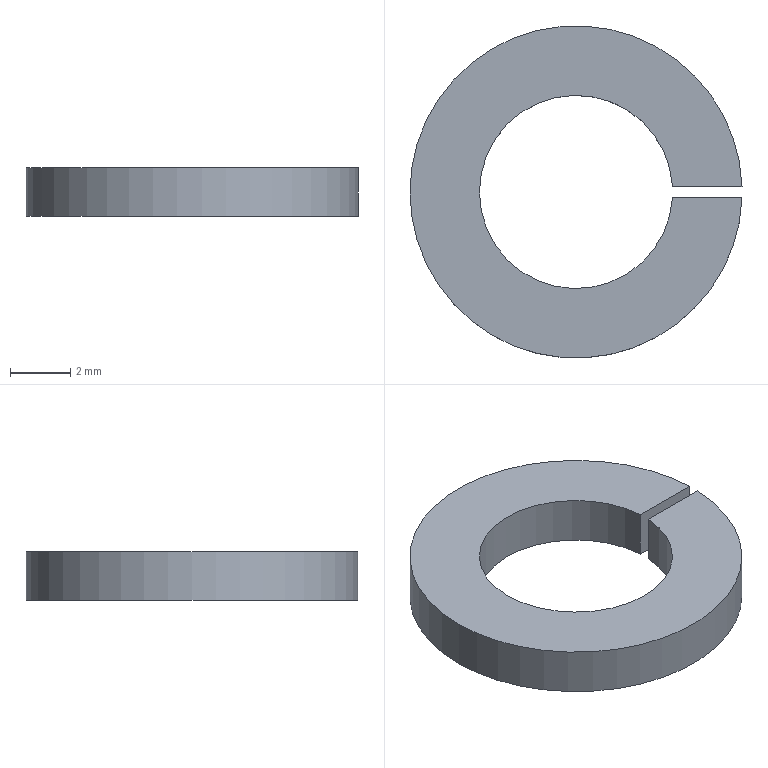Part | STEP file | GB93-1987 washer 6 | 1 solid | 6 faces | box 10.997 x 11 x 1.6 mm | volume 99.231 mm3 | plane 4 | cylinder 2 | commonest cylinder face diameters 6.4 x1 11 x1
STEP:
#1=CARTESIAN_POINT('',(5.497,0.1833,1.6));
#2=VERTEX_POINT('',#1);
#3=CARTESIAN_POINT('',(5.497,-0.1833,1.6));
#4=VERTEX_POINT('',#3);
#5=CARTESIAN_POINT('',(0.,0.,1.6));
#6=DIRECTION('',(0.,0.,1.));
#7=DIRECTION('',(1.,0.,0.));
#8=AXIS2_PLACEMENT_3D('',#5,#6,#7);
#9=CIRCLE('',#8,5.5);
#10=EDGE_CURVE('',#2,#4,#9,.T.);
#11=ORIENTED_EDGE('',*,*,#10,.T.);
#12=CARTESIAN_POINT('',(3.195,-0.1833,1.6));
#13=VERTEX_POINT('',#12);
#14=CARTESIAN_POINT('',(0.,-0.1833,1.6));
#15=DIRECTION('',(1.,0.,0.));
#16=VECTOR('',#15,1000.);
#17=LINE('',#14,#16);
#18=EDGE_CURVE('',#13,#4,#17,.T.);
#19=ORIENTED_EDGE('',*,*,#18,.F.);
#20=CARTESIAN_POINT('',(3.195,0.1833,1.6));
#21=VERTEX_POINT('',#20);
#22=CARTESIAN_POINT('',(0.,0.,1.6));
#23=DIRECTION('',(0.,0.,1.));
#24=DIRECTION('',(1.,0.,0.));
#25=AXIS2_PLACEMENT_3D('',#22,#23,#24);
#26=CIRCLE('',#25,3.2);
#27=EDGE_CURVE('',#21,#13,#26,.T.);
#28=ORIENTED_EDGE('',*,*,#27,.F.);
#29=CARTESIAN_POINT('',(0.,0.1833,1.6));
#30=DIRECTION('',(-1.,0.,0.));
#31=VECTOR('',#30,1000.);
#32=LINE('',#29,#31);
#33=EDGE_CURVE('',#2,#21,#32,.T.);
#34=ORIENTED_EDGE('',*,*,#33,.F.);
#35=EDGE_LOOP('',(#11,#19,#28,#34));
#36=FACE_OUTER_BOUND('',#35,.T.);
#37=CARTESIAN_POINT('',(0.,0.,1.6));
#38=DIRECTION('',(0.,0.,1.));
#39=DIRECTION('',(1.,0.,0.));
#40=AXIS2_PLACEMENT_3D('',#37,#38,#39);
#41=PLANE('',#40);
#42=ADVANCED_FACE('',(#36),#41,.T.);
#43=CARTESIAN_POINT('',(3.195,-0.1833,0.));
#44=VERTEX_POINT('',#43);
#45=CARTESIAN_POINT('',(5.497,-0.1833,0.));
#46=VERTEX_POINT('',#45);
#47=CARTESIAN_POINT('',(0.,-0.1833,0.));
#48=DIRECTION('',(1.,0.,0.));
#49=VECTOR('',#48,1000.);
#50=LINE('',#47,#49);
#51=EDGE_CURVE('',#44,#46,#50,.T.);
#52=ORIENTED_EDGE('',*,*,#51,.T.);
#53=CARTESIAN_POINT('',(5.497,0.1833,0.));
#54=VERTEX_POINT('',#53);
#55=CARTESIAN_POINT('',(0.,0.,0.));
#56=DIRECTION('',(0.,0.,1.));
#57=DIRECTION('',(1.,0.,0.));
#58=AXIS2_PLACEMENT_3D('',#55,#56,#57);
#59=CIRCLE('',#58,5.5);
#60=EDGE_CURVE('',#54,#46,#59,.T.);
#61=ORIENTED_EDGE('',*,*,#60,.F.);
#62=CARTESIAN_POINT('',(3.195,0.1833,0.));
#63=VERTEX_POINT('',#62);
#64=CARTESIAN_POINT('',(0.,0.1833,0.));
#65=DIRECTION('',(-1.,0.,0.));
#66=VECTOR('',#65,1000.);
#67=LINE('',#64,#66);
#68=EDGE_CURVE('',#54,#63,#67,.T.);
#69=ORIENTED_EDGE('',*,*,#68,.T.);
#70=CARTESIAN_POINT('',(0.,0.,0.));
#71=DIRECTION('',(0.,0.,1.));
#72=DIRECTION('',(1.,0.,0.));
#73=AXIS2_PLACEMENT_3D('',#70,#71,#72);
#74=CIRCLE('',#73,3.2);
#75=EDGE_CURVE('',#63,#44,#74,.T.);
#76=ORIENTED_EDGE('',*,*,#75,.T.);
#77=EDGE_LOOP('',(#52,#61,#69,#76));
#78=FACE_OUTER_BOUND('',#77,.T.);
#79=CARTESIAN_POINT('',(0.,0.,0.));
#80=DIRECTION('',(0.,0.,1.));
#81=DIRECTION('',(1.,0.,0.));
#82=AXIS2_PLACEMENT_3D('',#79,#80,#81);
#83=PLANE('',#82);
#84=ADVANCED_FACE('',(#78),#83,.F.);
#85=CARTESIAN_POINT('',(5.497,-0.1833,1.6));
#86=DIRECTION('',(0.,0.,-1.));
#87=VECTOR('',#86,1000.);
#88=LINE('',#85,#87);
#89=EDGE_CURVE('',#4,#46,#88,.T.);
#90=ORIENTED_EDGE('',*,*,#89,.F.);
#91=ORIENTED_EDGE('',*,*,#10,.F.);
#92=CARTESIAN_POINT('',(5.497,0.1833,1.6));
#93=DIRECTION('',(0.,0.,1.));
#94=VECTOR('',#93,1000.);
#95=LINE('',#92,#94);
#96=EDGE_CURVE('',#54,#2,#95,.T.);
#97=ORIENTED_EDGE('',*,*,#96,.F.);
#98=ORIENTED_EDGE('',*,*,#60,.T.);
#99=EDGE_LOOP('',(#90,#91,#97,#98));
#100=FACE_OUTER_BOUND('',#99,.T.);
#101=CARTESIAN_POINT('',(0.,0.,1.6));
#102=DIRECTION('',(0.,0.,-1.));
#103=DIRECTION('',(-1.,0.,0.));
#104=AXIS2_PLACEMENT_3D('',#101,#102,#103);
#105=CYLINDRICAL_SURFACE('',#104,5.5);
#106=ADVANCED_FACE('',(#100),#105,.T.);
#107=ORIENTED_EDGE('',*,*,#27,.T.);
#108=CARTESIAN_POINT('',(3.195,-0.1833,1.6));
#109=DIRECTION('',(0.,0.,-1.));
#110=VECTOR('',#109,1000.);
#111=LINE('',#108,#110);
#112=EDGE_CURVE('',#13,#44,#111,.T.);
#113=ORIENTED_EDGE('',*,*,#112,.T.);
#114=ORIENTED_EDGE('',*,*,#75,.F.);
#115=CARTESIAN_POINT('',(3.195,0.1833,1.6));
#116=DIRECTION('',(0.,0.,1.));
#117=VECTOR('',#116,1000.);
#118=LINE('',#115,#117);
#119=EDGE_CURVE('',#63,#21,#118,.T.);
#120=ORIENTED_EDGE('',*,*,#119,.T.);
#121=EDGE_LOOP('',(#107,#113,#114,#120));
#122=FACE_OUTER_BOUND('',#121,.T.);
#123=CARTESIAN_POINT('',(0.,0.,1.6));
#124=DIRECTION('',(0.,0.,-1.));
#125=DIRECTION('',(-1.,0.,0.));
#126=AXIS2_PLACEMENT_3D('',#123,#124,#125);
#127=CYLINDRICAL_SURFACE('',#126,3.2);
#128=ADVANCED_FACE('',(#122),#127,.F.);
#129=ORIENTED_EDGE('',*,*,#96,.T.);
#130=ORIENTED_EDGE('',*,*,#33,.T.);
#131=ORIENTED_EDGE('',*,*,#119,.F.);
#132=ORIENTED_EDGE('',*,*,#68,.F.);
#133=EDGE_LOOP('',(#129,#130,#131,#132));
#134=FACE_OUTER_BOUND('',#133,.T.);
#135=CARTESIAN_POINT('',(0.,0.1833,1.6));
#136=DIRECTION('',(0.,-1.,0.));
#137=DIRECTION('',(0.,0.,-1.));
#138=AXIS2_PLACEMENT_3D('',#135,#136,#137);
#139=PLANE('',#138);
#140=ADVANCED_FACE('',(#134),#139,.T.);
#141=ORIENTED_EDGE('',*,*,#89,.T.);
#142=ORIENTED_EDGE('',*,*,#51,.F.);
#143=ORIENTED_EDGE('',*,*,#112,.F.);
#144=ORIENTED_EDGE('',*,*,#18,.T.);
#145=EDGE_LOOP('',(#141,#142,#143,#144));
#146=FACE_OUTER_BOUND('',#145,.T.);
#147=CARTESIAN_POINT('',(0.,-0.1833,1.6));
#148=DIRECTION('',(0.,1.,0.));
#149=DIRECTION('',(0.,0.,1.));
#150=AXIS2_PLACEMENT_3D('',#147,#148,#149);
#151=PLANE('',#150);
#152=ADVANCED_FACE('',(#146),#151,.T.);
#153=CLOSED_SHELL('',(#42,#84,#106,#128,#140,#152));
#154=MANIFOLD_SOLID_BREP('',#153);
#155=CARTESIAN_POINT('',(0.,0.,0.));
#156=DIRECTION('',(0.,0.,1.));
#157=DIRECTION('',(1.,0.,0.));
#158=AXIS2_PLACEMENT_3D('',#155,#156,#157);
#159=(LENGTH_UNIT()NAMED_UNIT(*)SI_UNIT(.MILLI.,.METRE.));
#160=UNCERTAINTY_MEASURE_WITH_UNIT(LENGTH_MEASURE(0.00001),#159,'','');
#161=(NAMED_UNIT(*)PLANE_ANGLE_UNIT()SI_UNIT($,.RADIAN.));
#162=(NAMED_UNIT(*)SI_UNIT($,.STERADIAN.)SOLID_ANGLE_UNIT());
#163=(GEOMETRIC_REPRESENTATION_CONTEXT(3)GLOBAL_UNCERTAINTY_ASSIGNED_CONTEXT((#160))GLOBAL_UNIT_ASSIGNED_CONTEXT((#159,#161,#162))REPRESENTATION_CONTEXT('',''));
#164=ADVANCED_BREP_SHAPE_REPRESENTATION('',(#154,#158),#163);